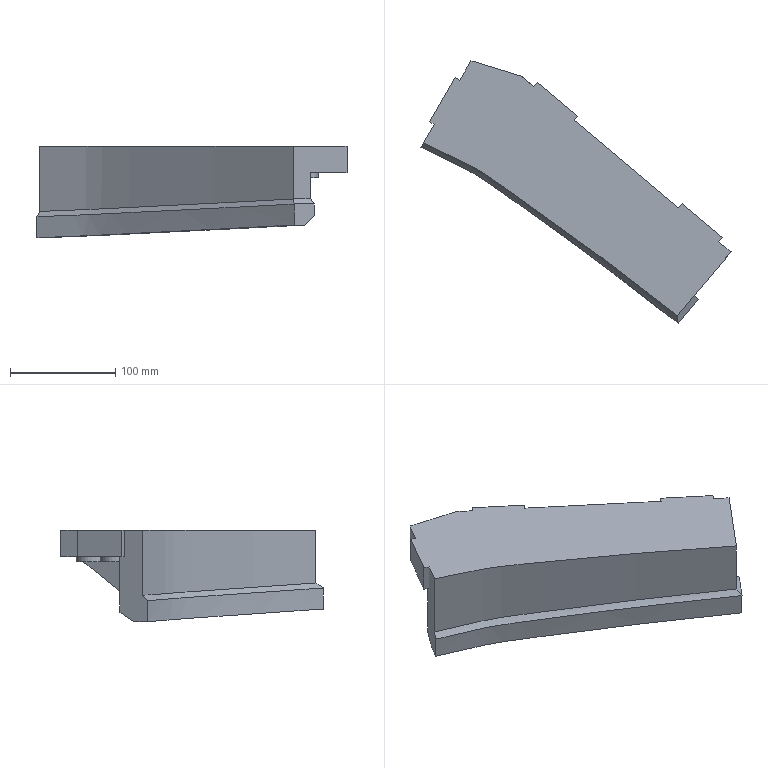Part | NX | features solid 2 | 1 solid | 39 faces | box 295.079 x 249.77 x 86.961 mm | volume 1166488 mm3 | plane 29 | spline 6 | cylinder 4 | commonest cylinder face diameters 30 x4